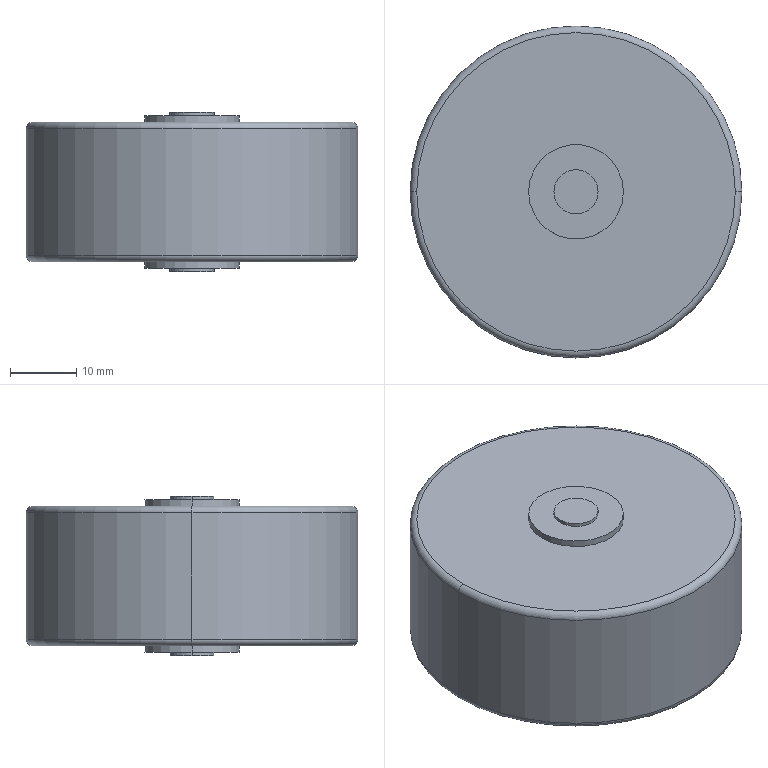Part | STEP file | CLGJ50_Uwheel | 1 solid | 20 faces | box 50 x 50 x 24 mm | volume 41522 mm3 | cylinder 10 | plane 6 | torus 4 | commonest cylinder face diameters 6.667 x4 14.286 x4 50 x2
STEP:
#1=CARTESIAN_POINT('',(3.333,0.,-12.));
#2=VERTEX_POINT('',#1);
#3=CARTESIAN_POINT('',(-3.333,0.,-12.));
#4=VERTEX_POINT('',#3);
#5=CARTESIAN_POINT('',(0.,0.,-12.));
#6=DIRECTION('',(0.,0.,1.));
#7=DIRECTION('',(1.,0.,0.));
#8=AXIS2_PLACEMENT_3D('',#5,#6,#7);
#9=CIRCLE('',#8,3.333);
#10=EDGE_CURVE('',#2,#4,#9,.T.);
#11=ORIENTED_EDGE('',*,*,#10,.T.);
#12=CARTESIAN_POINT('',(-3.333,0.,-11.5));
#13=VERTEX_POINT('',#12);
#14=CARTESIAN_POINT('',(-3.333,0.,-12.));
#15=DIRECTION('',(0.,0.,1.));
#16=VECTOR('',#15,1000.);
#17=LINE('',#14,#16);
#18=EDGE_CURVE('',#4,#13,#17,.T.);
#19=ORIENTED_EDGE('',*,*,#18,.T.);
#20=CARTESIAN_POINT('',(3.333,0.,-11.5));
#21=VERTEX_POINT('',#20);
#22=CARTESIAN_POINT('',(0.,0.,-11.5));
#23=DIRECTION('',(0.,0.,1.));
#24=DIRECTION('',(1.,0.,0.));
#25=AXIS2_PLACEMENT_3D('',#22,#23,#24);
#26=CIRCLE('',#25,3.333);
#27=EDGE_CURVE('',#21,#13,#26,.T.);
#28=ORIENTED_EDGE('',*,*,#27,.F.);
#29=CARTESIAN_POINT('',(3.333,0.,-12.));
#30=DIRECTION('',(0.,0.,1.));
#31=VECTOR('',#30,1000.);
#32=LINE('',#29,#31);
#33=EDGE_CURVE('',#2,#21,#32,.T.);
#34=ORIENTED_EDGE('',*,*,#33,.F.);
#35=EDGE_LOOP('',(#11,#19,#28,#34));
#36=FACE_OUTER_BOUND('',#35,.T.);
#37=CARTESIAN_POINT('',(0.,0.,-12.));
#38=DIRECTION('',(0.,0.,1.));
#39=DIRECTION('',(1.,0.,0.));
#40=AXIS2_PLACEMENT_3D('',#37,#38,#39);
#41=CYLINDRICAL_SURFACE('',#40,3.333);
#42=ADVANCED_FACE('',(#36),#41,.T.);
#43=CARTESIAN_POINT('',(7.143,0.,-11.5));
#44=VERTEX_POINT('',#43);
#45=CARTESIAN_POINT('',(-7.143,0.,-11.5));
#46=VERTEX_POINT('',#45);
#47=CARTESIAN_POINT('',(0.,0.,-11.5));
#48=DIRECTION('',(0.,0.,1.));
#49=DIRECTION('',(1.,0.,0.));
#50=AXIS2_PLACEMENT_3D('',#47,#48,#49);
#51=CIRCLE('',#50,7.143);
#52=EDGE_CURVE('',#44,#46,#51,.T.);
#53=ORIENTED_EDGE('',*,*,#52,.T.);
#54=CARTESIAN_POINT('',(-7.143,0.,-10.5));
#55=VERTEX_POINT('',#54);
#56=CARTESIAN_POINT('',(-7.143,0.,-12.));
#57=DIRECTION('',(0.,0.,1.));
#58=VECTOR('',#57,1000.);
#59=LINE('',#56,#58);
#60=EDGE_CURVE('',#46,#55,#59,.T.);
#61=ORIENTED_EDGE('',*,*,#60,.T.);
#62=CARTESIAN_POINT('',(7.143,0.,-10.5));
#63=VERTEX_POINT('',#62);
#64=CARTESIAN_POINT('',(0.,0.,-10.5));
#65=DIRECTION('',(0.,0.,1.));
#66=DIRECTION('',(1.,0.,0.));
#67=AXIS2_PLACEMENT_3D('',#64,#65,#66);
#68=CIRCLE('',#67,7.143);
#69=EDGE_CURVE('',#63,#55,#68,.T.);
#70=ORIENTED_EDGE('',*,*,#69,.F.);
#71=CARTESIAN_POINT('',(7.143,0.,-12.));
#72=DIRECTION('',(0.,0.,1.));
#73=VECTOR('',#72,1000.);
#74=LINE('',#71,#73);
#75=EDGE_CURVE('',#44,#63,#74,.T.);
#76=ORIENTED_EDGE('',*,*,#75,.F.);
#77=EDGE_LOOP('',(#53,#61,#70,#76));
#78=FACE_OUTER_BOUND('',#77,.T.);
#79=CARTESIAN_POINT('',(0.,0.,-12.));
#80=DIRECTION('',(0.,0.,1.));
#81=DIRECTION('',(1.,0.,0.));
#82=AXIS2_PLACEMENT_3D('',#79,#80,#81);
#83=CYLINDRICAL_SURFACE('',#82,7.143);
#84=ADVANCED_FACE('',(#78),#83,.T.);
#85=CARTESIAN_POINT('',(24.,0.,-10.5));
#86=VERTEX_POINT('',#85);
#87=CARTESIAN_POINT('',(-24.,0.,-10.5));
#88=VERTEX_POINT('',#87);
#89=CARTESIAN_POINT('',(0.,0.,-10.5));
#90=DIRECTION('',(0.,0.,1.));
#91=DIRECTION('',(1.,0.,0.));
#92=AXIS2_PLACEMENT_3D('',#89,#90,#91);
#93=CIRCLE('',#92,24.);
#94=EDGE_CURVE('',#86,#88,#93,.T.);
#95=ORIENTED_EDGE('',*,*,#94,.T.);
#96=CARTESIAN_POINT('',(-25.,0.,-9.5));
#97=VERTEX_POINT('',#96);
#98=CARTESIAN_POINT('',(-24.,0.,-9.5));
#99=DIRECTION('',(0.,1.,0.));
#100=DIRECTION('',(-1.,0.,0.));
#101=AXIS2_PLACEMENT_3D('',#98,#99,#100);
#102=CIRCLE('',#101,1.);
#103=EDGE_CURVE('',#88,#97,#102,.T.);
#104=ORIENTED_EDGE('',*,*,#103,.T.);
#105=CARTESIAN_POINT('',(25.,0.,-9.5));
#106=VERTEX_POINT('',#105);
#107=CARTESIAN_POINT('',(0.,0.,-9.5));
#108=DIRECTION('',(0.,0.,1.));
#109=DIRECTION('',(1.,0.,0.));
#110=AXIS2_PLACEMENT_3D('',#107,#108,#109);
#111=CIRCLE('',#110,25.);
#112=EDGE_CURVE('',#106,#97,#111,.T.);
#113=ORIENTED_EDGE('',*,*,#112,.F.);
#114=CARTESIAN_POINT('',(24.,0.,-9.5));
#115=DIRECTION('',(0.,-1.,0.));
#116=DIRECTION('',(0.,0.,-1.));
#117=AXIS2_PLACEMENT_3D('',#114,#115,#116);
#118=CIRCLE('',#117,1.);
#119=EDGE_CURVE('',#86,#106,#118,.T.);
#120=ORIENTED_EDGE('',*,*,#119,.F.);
#121=EDGE_LOOP('',(#95,#104,#113,#120));
#122=FACE_OUTER_BOUND('',#121,.T.);
#123=CARTESIAN_POINT('',(0.,0.,-9.5));
#124=DIRECTION('',(0.,0.,1.));
#125=DIRECTION('',(1.,0.,0.));
#126=AXIS2_PLACEMENT_3D('',#123,#124,#125);
#127=TOROIDAL_SURFACE('',#126,24.,1.);
#128=ADVANCED_FACE('',(#122),#127,.T.);
#129=ORIENTED_EDGE('',*,*,#112,.T.);
#130=CARTESIAN_POINT('',(-25.,0.,9.5));
#131=VERTEX_POINT('',#130);
#132=CARTESIAN_POINT('',(-25.,0.,-12.));
#133=DIRECTION('',(0.,0.,1.));
#134=VECTOR('',#133,1000.);
#135=LINE('',#132,#134);
#136=EDGE_CURVE('',#97,#131,#135,.T.);
#137=ORIENTED_EDGE('',*,*,#136,.T.);
#138=CARTESIAN_POINT('',(25.,0.,9.5));
#139=VERTEX_POINT('',#138);
#140=CARTESIAN_POINT('',(0.,0.,9.5));
#141=DIRECTION('',(0.,0.,1.));
#142=DIRECTION('',(1.,0.,0.));
#143=AXIS2_PLACEMENT_3D('',#140,#141,#142);
#144=CIRCLE('',#143,25.);
#145=EDGE_CURVE('',#139,#131,#144,.T.);
#146=ORIENTED_EDGE('',*,*,#145,.F.);
#147=CARTESIAN_POINT('',(25.,0.,-12.));
#148=DIRECTION('',(0.,0.,1.));
#149=VECTOR('',#148,1000.);
#150=LINE('',#147,#149);
#151=EDGE_CURVE('',#106,#139,#150,.T.);
#152=ORIENTED_EDGE('',*,*,#151,.F.);
#153=EDGE_LOOP('',(#129,#137,#146,#152));
#154=FACE_OUTER_BOUND('',#153,.T.);
#155=CARTESIAN_POINT('',(0.,0.,-12.));
#156=DIRECTION('',(0.,0.,1.));
#157=DIRECTION('',(1.,0.,0.));
#158=AXIS2_PLACEMENT_3D('',#155,#156,#157);
#159=CYLINDRICAL_SURFACE('',#158,25.);
#160=ADVANCED_FACE('',(#154),#159,.T.);
#161=ORIENTED_EDGE('',*,*,#145,.T.);
#162=CARTESIAN_POINT('',(-24.,0.,10.5));
#163=VERTEX_POINT('',#162);
#164=CARTESIAN_POINT('',(-24.,0.,9.5));
#165=DIRECTION('',(0.,1.,0.));
#166=DIRECTION('',(-1.,0.,0.));
#167=AXIS2_PLACEMENT_3D('',#164,#165,#166);
#168=CIRCLE('',#167,1.);
#169=EDGE_CURVE('',#131,#163,#168,.T.);
#170=ORIENTED_EDGE('',*,*,#169,.T.);
#171=CARTESIAN_POINT('',(24.,0.,10.5));
#172=VERTEX_POINT('',#171);
#173=CARTESIAN_POINT('',(0.,0.,10.5));
#174=DIRECTION('',(0.,0.,1.));
#175=DIRECTION('',(1.,0.,0.));
#176=AXIS2_PLACEMENT_3D('',#173,#174,#175);
#177=CIRCLE('',#176,24.);
#178=EDGE_CURVE('',#172,#163,#177,.T.);
#179=ORIENTED_EDGE('',*,*,#178,.F.);
#180=CARTESIAN_POINT('',(24.,0.,9.5));
#181=DIRECTION('',(0.,-1.,0.));
#182=DIRECTION('',(0.,0.,-1.));
#183=AXIS2_PLACEMENT_3D('',#180,#181,#182);
#184=CIRCLE('',#183,1.);
#185=EDGE_CURVE('',#139,#172,#184,.T.);
#186=ORIENTED_EDGE('',*,*,#185,.F.);
#187=EDGE_LOOP('',(#161,#170,#179,#186));
#188=FACE_OUTER_BOUND('',#187,.T.);
#189=CARTESIAN_POINT('',(0.,0.,9.5));
#190=DIRECTION('',(0.,0.,1.));
#191=DIRECTION('',(1.,0.,0.));
#192=AXIS2_PLACEMENT_3D('',#189,#190,#191);
#193=TOROIDAL_SURFACE('',#192,24.,1.);
#194=ADVANCED_FACE('',(#188),#193,.T.);
#195=CARTESIAN_POINT('',(7.143,0.,10.5));
#196=VERTEX_POINT('',#195);
#197=CARTESIAN_POINT('',(-7.143,0.,10.5));
#198=VERTEX_POINT('',#197);
#199=CARTESIAN_POINT('',(0.,0.,10.5));
#200=DIRECTION('',(0.,0.,1.));
#201=DIRECTION('',(1.,0.,0.));
#202=AXIS2_PLACEMENT_3D('',#199,#200,#201);
#203=CIRCLE('',#202,7.143);
#204=EDGE_CURVE('',#196,#198,#203,.T.);
#205=ORIENTED_EDGE('',*,*,#204,.T.);
#206=CARTESIAN_POINT('',(-7.143,0.,11.5));
#207=VERTEX_POINT('',#206);
#208=CARTESIAN_POINT('',(-7.143,0.,-12.));
#209=DIRECTION('',(0.,0.,1.));
#210=VECTOR('',#209,1000.);
#211=LINE('',#208,#210);
#212=EDGE_CURVE('',#198,#207,#211,.T.);
#213=ORIENTED_EDGE('',*,*,#212,.T.);
#214=CARTESIAN_POINT('',(7.143,0.,11.5));
#215=VERTEX_POINT('',#214);
#216=CARTESIAN_POINT('',(0.,0.,11.5));
#217=DIRECTION('',(0.,0.,1.));
#218=DIRECTION('',(1.,0.,0.));
#219=AXIS2_PLACEMENT_3D('',#216,#217,#218);
#220=CIRCLE('',#219,7.143);
#221=EDGE_CURVE('',#215,#207,#220,.T.);
#222=ORIENTED_EDGE('',*,*,#221,.F.);
#223=CARTESIAN_POINT('',(7.143,0.,-12.));
#224=DIRECTION('',(0.,0.,1.));
#225=VECTOR('',#224,1000.);
#226=LINE('',#223,#225);
#227=EDGE_CURVE('',#196,#215,#226,.T.);
#228=ORIENTED_EDGE('',*,*,#227,.F.);
#229=EDGE_LOOP('',(#205,#213,#222,#228));
#230=FACE_OUTER_BOUND('',#229,.T.);
#231=CARTESIAN_POINT('',(0.,0.,-12.));
#232=DIRECTION('',(0.,0.,1.));
#233=DIRECTION('',(1.,0.,0.));
#234=AXIS2_PLACEMENT_3D('',#231,#232,#233);
#235=CYLINDRICAL_SURFACE('',#234,7.143);
#236=ADVANCED_FACE('',(#230),#235,.T.);
#237=CARTESIAN_POINT('',(3.333,0.,11.5));
#238=VERTEX_POINT('',#237);
#239=CARTESIAN_POINT('',(-3.333,0.,11.5));
#240=VERTEX_POINT('',#239);
#241=CARTESIAN_POINT('',(0.,0.,11.5));
#242=DIRECTION('',(0.,0.,1.));
#243=DIRECTION('',(1.,0.,0.));
#244=AXIS2_PLACEMENT_3D('',#241,#242,#243);
#245=CIRCLE('',#244,3.333);
#246=EDGE_CURVE('',#238,#240,#245,.T.);
#247=ORIENTED_EDGE('',*,*,#246,.T.);
#248=CARTESIAN_POINT('',(-3.333,0.,12.));
#249=VERTEX_POINT('',#248);
#250=CARTESIAN_POINT('',(-3.333,0.,-12.));
#251=DIRECTION('',(0.,0.,1.));
#252=VECTOR('',#251,1000.);
#253=LINE('',#250,#252);
#254=EDGE_CURVE('',#240,#249,#253,.T.);
#255=ORIENTED_EDGE('',*,*,#254,.T.);
#256=CARTESIAN_POINT('',(3.333,0.,12.));
#257=VERTEX_POINT('',#256);
#258=CARTESIAN_POINT('',(0.,0.,12.));
#259=DIRECTION('',(0.,0.,1.));
#260=DIRECTION('',(1.,0.,0.));
#261=AXIS2_PLACEMENT_3D('',#258,#259,#260);
#262=CIRCLE('',#261,3.333);
#263=EDGE_CURVE('',#257,#249,#262,.T.);
#264=ORIENTED_EDGE('',*,*,#263,.F.);
#265=CARTESIAN_POINT('',(3.333,0.,-12.));
#266=DIRECTION('',(0.,0.,1.));
#267=VECTOR('',#266,1000.);
#268=LINE('',#265,#267);
#269=EDGE_CURVE('',#238,#257,#268,.T.);
#270=ORIENTED_EDGE('',*,*,#269,.F.);
#271=EDGE_LOOP('',(#247,#255,#264,#270));
#272=FACE_OUTER_BOUND('',#271,.T.);
#273=CARTESIAN_POINT('',(0.,0.,-12.));
#274=DIRECTION('',(0.,0.,1.));
#275=DIRECTION('',(1.,0.,0.));
#276=AXIS2_PLACEMENT_3D('',#273,#274,#275);
#277=CYLINDRICAL_SURFACE('',#276,3.333);
#278=ADVANCED_FACE('',(#272),#277,.T.);
#279=ORIENTED_EDGE('',*,*,#263,.T.);
#280=CARTESIAN_POINT('',(0.,0.,12.));
#281=DIRECTION('',(0.,0.,1.));
#282=DIRECTION('',(1.,0.,0.));
#283=AXIS2_PLACEMENT_3D('',#280,#281,#282);
#284=CIRCLE('',#283,3.333);
#285=EDGE_CURVE('',#249,#257,#284,.T.);
#286=ORIENTED_EDGE('',*,*,#285,.T.);
#287=EDGE_LOOP('',(#279,#286));
#288=FACE_OUTER_BOUND('',#287,.T.);
#289=CARTESIAN_POINT('',(0.,0.,12.));
#290=DIRECTION('',(0.,0.,-1.));
#291=DIRECTION('',(-1.,0.,0.));
#292=AXIS2_PLACEMENT_3D('',#289,#290,#291);
#293=PLANE('',#292);
#294=ADVANCED_FACE('',(#288),#293,.F.);
#295=ORIENTED_EDGE('',*,*,#254,.F.);
#296=CARTESIAN_POINT('',(0.,0.,11.5));
#297=DIRECTION('',(0.,0.,1.));
#298=DIRECTION('',(1.,0.,0.));
#299=AXIS2_PLACEMENT_3D('',#296,#297,#298);
#300=CIRCLE('',#299,3.333);
#301=EDGE_CURVE('',#240,#238,#300,.T.);
#302=ORIENTED_EDGE('',*,*,#301,.T.);
#303=ORIENTED_EDGE('',*,*,#269,.T.);
#304=ORIENTED_EDGE('',*,*,#285,.F.);
#305=EDGE_LOOP('',(#295,#302,#303,#304));
#306=FACE_OUTER_BOUND('',#305,.T.);
#307=CARTESIAN_POINT('',(0.,0.,-12.));
#308=DIRECTION('',(0.,0.,1.));
#309=DIRECTION('',(1.,0.,0.));
#310=AXIS2_PLACEMENT_3D('',#307,#308,#309);
#311=CYLINDRICAL_SURFACE('',#310,3.333);
#312=ADVANCED_FACE('',(#306),#311,.T.);
#313=ORIENTED_EDGE('',*,*,#246,.F.);
#314=ORIENTED_EDGE('',*,*,#301,.F.);
#315=EDGE_LOOP('',(#313,#314));
#316=FACE_BOUND('',#315,.T.);
#317=ORIENTED_EDGE('',*,*,#221,.T.);
#318=CARTESIAN_POINT('',(0.,0.,11.5));
#319=DIRECTION('',(0.,0.,1.));
#320=DIRECTION('',(1.,0.,0.));
#321=AXIS2_PLACEMENT_3D('',#318,#319,#320);
#322=CIRCLE('',#321,7.143);
#323=EDGE_CURVE('',#207,#215,#322,.T.);
#324=ORIENTED_EDGE('',*,*,#323,.T.);
#325=EDGE_LOOP('',(#317,#324));
#326=FACE_OUTER_BOUND('',#325,.T.);
#327=CARTESIAN_POINT('',(0.,3.333,11.5));
#328=DIRECTION('',(0.,0.,-1.));
#329=DIRECTION('',(-1.,0.,0.));
#330=AXIS2_PLACEMENT_3D('',#327,#328,#329);
#331=PLANE('',#330);
#332=ADVANCED_FACE('',(#316,#326),#331,.F.);
#333=ORIENTED_EDGE('',*,*,#212,.F.);
#334=CARTESIAN_POINT('',(0.,0.,10.5));
#335=DIRECTION('',(0.,0.,1.));
#336=DIRECTION('',(1.,0.,0.));
#337=AXIS2_PLACEMENT_3D('',#334,#335,#336);
#338=CIRCLE('',#337,7.143);
#339=EDGE_CURVE('',#198,#196,#338,.T.);
#340=ORIENTED_EDGE('',*,*,#339,.T.);
#341=ORIENTED_EDGE('',*,*,#227,.T.);
#342=ORIENTED_EDGE('',*,*,#323,.F.);
#343=EDGE_LOOP('',(#333,#340,#341,#342));
#344=FACE_OUTER_BOUND('',#343,.T.);
#345=CARTESIAN_POINT('',(0.,0.,-12.));
#346=DIRECTION('',(0.,0.,1.));
#347=DIRECTION('',(1.,0.,0.));
#348=AXIS2_PLACEMENT_3D('',#345,#346,#347);
#349=CYLINDRICAL_SURFACE('',#348,7.143);
#350=ADVANCED_FACE('',(#344),#349,.T.);
#351=ORIENTED_EDGE('',*,*,#204,.F.);
#352=ORIENTED_EDGE('',*,*,#339,.F.);
#353=EDGE_LOOP('',(#351,#352));
#354=FACE_BOUND('',#353,.T.);
#355=ORIENTED_EDGE('',*,*,#178,.T.);
#356=CARTESIAN_POINT('',(0.,0.,10.5));
#357=DIRECTION('',(0.,0.,1.));
#358=DIRECTION('',(1.,0.,0.));
#359=AXIS2_PLACEMENT_3D('',#356,#357,#358);
#360=CIRCLE('',#359,24.);
#361=EDGE_CURVE('',#163,#172,#360,.T.);
#362=ORIENTED_EDGE('',*,*,#361,.T.);
#363=EDGE_LOOP('',(#355,#362));
#364=FACE_OUTER_BOUND('',#363,.T.);
#365=CARTESIAN_POINT('',(0.,7.143,10.5));
#366=DIRECTION('',(0.,0.,-1.));
#367=DIRECTION('',(-1.,0.,0.));
#368=AXIS2_PLACEMENT_3D('',#365,#366,#367);
#369=PLANE('',#368);
#370=ADVANCED_FACE('',(#354,#364),#369,.F.);
#371=ORIENTED_EDGE('',*,*,#169,.F.);
#372=CARTESIAN_POINT('',(0.,0.,9.5));
#373=DIRECTION('',(0.,0.,1.));
#374=DIRECTION('',(1.,0.,0.));
#375=AXIS2_PLACEMENT_3D('',#372,#373,#374);
#376=CIRCLE('',#375,25.);
#377=EDGE_CURVE('',#131,#139,#376,.T.);
#378=ORIENTED_EDGE('',*,*,#377,.T.);
#379=ORIENTED_EDGE('',*,*,#185,.T.);
#380=ORIENTED_EDGE('',*,*,#361,.F.);
#381=EDGE_LOOP('',(#371,#378,#379,#380));
#382=FACE_OUTER_BOUND('',#381,.T.);
#383=CARTESIAN_POINT('',(0.,0.,9.5));
#384=DIRECTION('',(0.,0.,1.));
#385=DIRECTION('',(1.,0.,0.));
#386=AXIS2_PLACEMENT_3D('',#383,#384,#385);
#387=TOROIDAL_SURFACE('',#386,24.,1.);
#388=ADVANCED_FACE('',(#382),#387,.T.);
#389=ORIENTED_EDGE('',*,*,#136,.F.);
#390=CARTESIAN_POINT('',(0.,0.,-9.5));
#391=DIRECTION('',(0.,0.,1.));
#392=DIRECTION('',(1.,0.,0.));
#393=AXIS2_PLACEMENT_3D('',#390,#391,#392);
#394=CIRCLE('',#393,25.);
#395=EDGE_CURVE('',#97,#106,#394,.T.);
#396=ORIENTED_EDGE('',*,*,#395,.T.);
#397=ORIENTED_EDGE('',*,*,#151,.T.);
#398=ORIENTED_EDGE('',*,*,#377,.F.);
#399=EDGE_LOOP('',(#389,#396,#397,#398));
#400=FACE_OUTER_BOUND('',#399,.T.);
#401=CARTESIAN_POINT('',(0.,0.,-12.));
#402=DIRECTION('',(0.,0.,1.));
#403=DIRECTION('',(1.,0.,0.));
#404=AXIS2_PLACEMENT_3D('',#401,#402,#403);
#405=CYLINDRICAL_SURFACE('',#404,25.);
#406=ADVANCED_FACE('',(#400),#405,.T.);
#407=ORIENTED_EDGE('',*,*,#103,.F.);
#408=CARTESIAN_POINT('',(0.,0.,-10.5));
#409=DIRECTION('',(0.,0.,1.));
#410=DIRECTION('',(1.,0.,0.));
#411=AXIS2_PLACEMENT_3D('',#408,#409,#410);
#412=CIRCLE('',#411,24.);
#413=EDGE_CURVE('',#88,#86,#412,.T.);
#414=ORIENTED_EDGE('',*,*,#413,.T.);
#415=ORIENTED_EDGE('',*,*,#119,.T.);
#416=ORIENTED_EDGE('',*,*,#395,.F.);
#417=EDGE_LOOP('',(#407,#414,#415,#416));
#418=FACE_OUTER_BOUND('',#417,.T.);
#419=CARTESIAN_POINT('',(0.,0.,-9.5));
#420=DIRECTION('',(0.,0.,1.));
#421=DIRECTION('',(1.,0.,0.));
#422=AXIS2_PLACEMENT_3D('',#419,#420,#421);
#423=TOROIDAL_SURFACE('',#422,24.,1.);
#424=ADVANCED_FACE('',(#418),#423,.T.);
#425=ORIENTED_EDGE('',*,*,#94,.F.);
#426=ORIENTED_EDGE('',*,*,#413,.F.);
#427=EDGE_LOOP('',(#425,#426));
#428=FACE_OUTER_BOUND('',#427,.T.);
#429=ORIENTED_EDGE('',*,*,#69,.T.);
#430=CARTESIAN_POINT('',(0.,0.,-10.5));
#431=DIRECTION('',(0.,0.,1.));
#432=DIRECTION('',(1.,0.,0.));
#433=AXIS2_PLACEMENT_3D('',#430,#431,#432);
#434=CIRCLE('',#433,7.143);
#435=EDGE_CURVE('',#55,#63,#434,.T.);
#436=ORIENTED_EDGE('',*,*,#435,.T.);
#437=EDGE_LOOP('',(#429,#436));
#438=FACE_BOUND('',#437,.T.);
#439=CARTESIAN_POINT('',(0.,24.,-10.5));
#440=DIRECTION('',(0.,0.,1.));
#441=DIRECTION('',(1.,0.,0.));
#442=AXIS2_PLACEMENT_3D('',#439,#440,#441);
#443=PLANE('',#442);
#444=ADVANCED_FACE('',(#428,#438),#443,.F.);
#445=ORIENTED_EDGE('',*,*,#60,.F.);
#446=CARTESIAN_POINT('',(0.,0.,-11.5));
#447=DIRECTION('',(0.,0.,1.));
#448=DIRECTION('',(1.,0.,0.));
#449=AXIS2_PLACEMENT_3D('',#446,#447,#448);
#450=CIRCLE('',#449,7.143);
#451=EDGE_CURVE('',#46,#44,#450,.T.);
#452=ORIENTED_EDGE('',*,*,#451,.T.);
#453=ORIENTED_EDGE('',*,*,#75,.T.);
#454=ORIENTED_EDGE('',*,*,#435,.F.);
#455=EDGE_LOOP('',(#445,#452,#453,#454));
#456=FACE_OUTER_BOUND('',#455,.T.);
#457=CARTESIAN_POINT('',(0.,0.,-12.));
#458=DIRECTION('',(0.,0.,1.));
#459=DIRECTION('',(1.,0.,0.));
#460=AXIS2_PLACEMENT_3D('',#457,#458,#459);
#461=CYLINDRICAL_SURFACE('',#460,7.143);
#462=ADVANCED_FACE('',(#456),#461,.T.);
#463=ORIENTED_EDGE('',*,*,#52,.F.);
#464=ORIENTED_EDGE('',*,*,#451,.F.);
#465=EDGE_LOOP('',(#463,#464));
#466=FACE_OUTER_BOUND('',#465,.T.);
#467=ORIENTED_EDGE('',*,*,#27,.T.);
#468=CARTESIAN_POINT('',(0.,0.,-11.5));
#469=DIRECTION('',(0.,0.,1.));
#470=DIRECTION('',(1.,0.,0.));
#471=AXIS2_PLACEMENT_3D('',#468,#469,#470);
#472=CIRCLE('',#471,3.333);
#473=EDGE_CURVE('',#13,#21,#472,.T.);
#474=ORIENTED_EDGE('',*,*,#473,.T.);
#475=EDGE_LOOP('',(#467,#474));
#476=FACE_BOUND('',#475,.T.);
#477=CARTESIAN_POINT('',(0.,7.143,-11.5));
#478=DIRECTION('',(0.,0.,1.));
#479=DIRECTION('',(1.,0.,0.));
#480=AXIS2_PLACEMENT_3D('',#477,#478,#479);
#481=PLANE('',#480);
#482=ADVANCED_FACE('',(#466,#476),#481,.F.);
#483=ORIENTED_EDGE('',*,*,#18,.F.);
#484=CARTESIAN_POINT('',(0.,0.,-12.));
#485=DIRECTION('',(0.,0.,1.));
#486=DIRECTION('',(1.,0.,0.));
#487=AXIS2_PLACEMENT_3D('',#484,#485,#486);
#488=CIRCLE('',#487,3.333);
#489=EDGE_CURVE('',#4,#2,#488,.T.);
#490=ORIENTED_EDGE('',*,*,#489,.T.);
#491=ORIENTED_EDGE('',*,*,#33,.T.);
#492=ORIENTED_EDGE('',*,*,#473,.F.);
#493=EDGE_LOOP('',(#483,#490,#491,#492));
#494=FACE_OUTER_BOUND('',#493,.T.);
#495=CARTESIAN_POINT('',(0.,0.,-12.));
#496=DIRECTION('',(0.,0.,1.));
#497=DIRECTION('',(1.,0.,0.));
#498=AXIS2_PLACEMENT_3D('',#495,#496,#497);
#499=CYLINDRICAL_SURFACE('',#498,3.333);
#500=ADVANCED_FACE('',(#494),#499,.T.);
#501=ORIENTED_EDGE('',*,*,#10,.F.);
#502=ORIENTED_EDGE('',*,*,#489,.F.);
#503=EDGE_LOOP('',(#501,#502));
#504=FACE_OUTER_BOUND('',#503,.T.);
#505=CARTESIAN_POINT('',(0.,3.333,-12.));
#506=DIRECTION('',(0.,0.,1.));
#507=DIRECTION('',(1.,0.,0.));
#508=AXIS2_PLACEMENT_3D('',#505,#506,#507);
#509=PLANE('',#508);
#510=ADVANCED_FACE('',(#504),#509,.F.);
#511=CLOSED_SHELL('',(#42,#84,#128,#160,#194,#236,#278,#294,#312,#332,#350,#370,#388,#406,#424,#444,#462,#482,#500,#510));
#512=MANIFOLD_SOLID_BREP('',#511);
#513=CARTESIAN_POINT('',(0.,0.,0.));
#514=DIRECTION('',(0.,0.,1.));
#515=DIRECTION('',(1.,0.,0.));
#516=AXIS2_PLACEMENT_3D('',#513,#514,#515);
#517=(LENGTH_UNIT()NAMED_UNIT(*)SI_UNIT(.MILLI.,.METRE.));
#518=UNCERTAINTY_MEASURE_WITH_UNIT(LENGTH_MEASURE(0.00001),#517,'','');
#519=(NAMED_UNIT(*)PLANE_ANGLE_UNIT()SI_UNIT($,.RADIAN.));
#520=(NAMED_UNIT(*)SI_UNIT($,.STERADIAN.)SOLID_ANGLE_UNIT());
#521=(GEOMETRIC_REPRESENTATION_CONTEXT(3)GLOBAL_UNCERTAINTY_ASSIGNED_CONTEXT((#518))GLOBAL_UNIT_ASSIGNED_CONTEXT((#517,#519,#520))REPRESENTATION_CONTEXT('',''));
#522=ADVANCED_BREP_SHAPE_REPRESENTATION('',(#512,#516),#521);